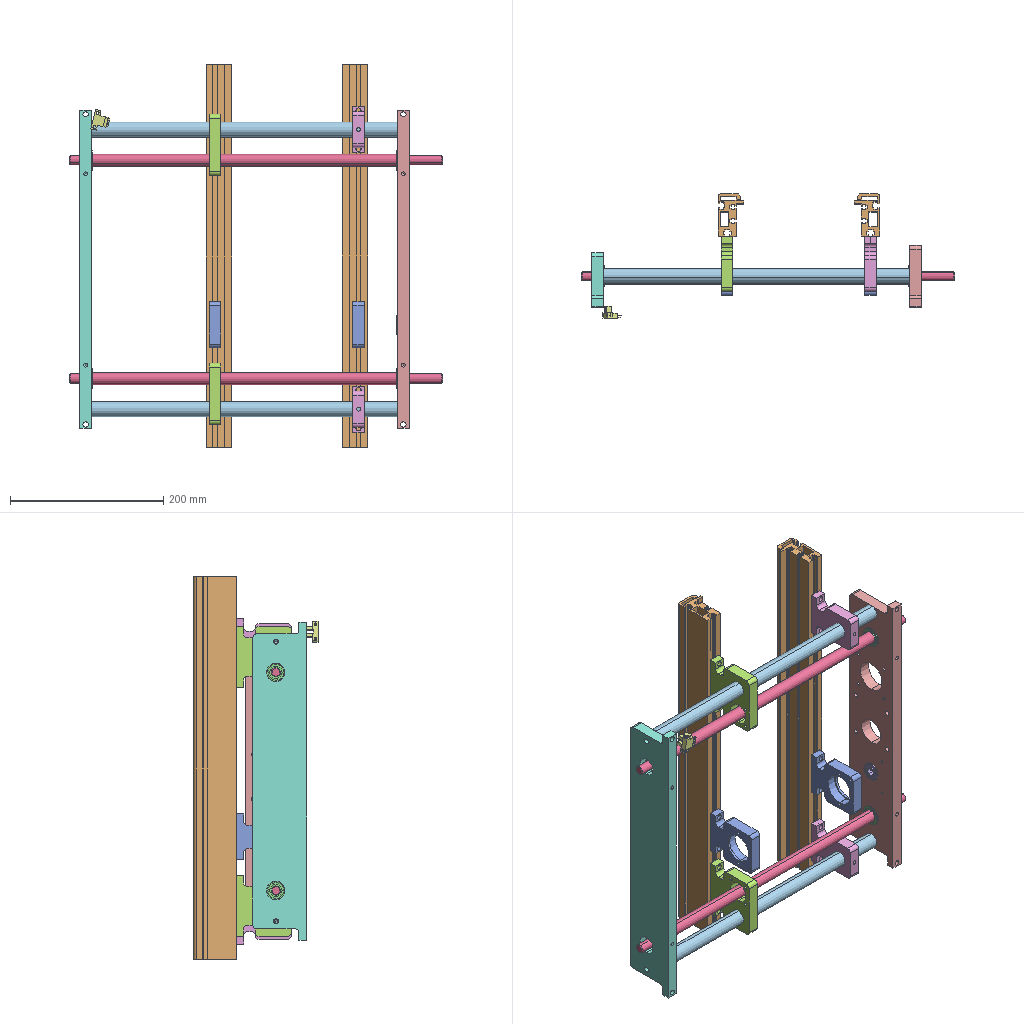Assembly | SolidWorks | 11 different items | 20 placed | box 487 x 162 x 500 mm
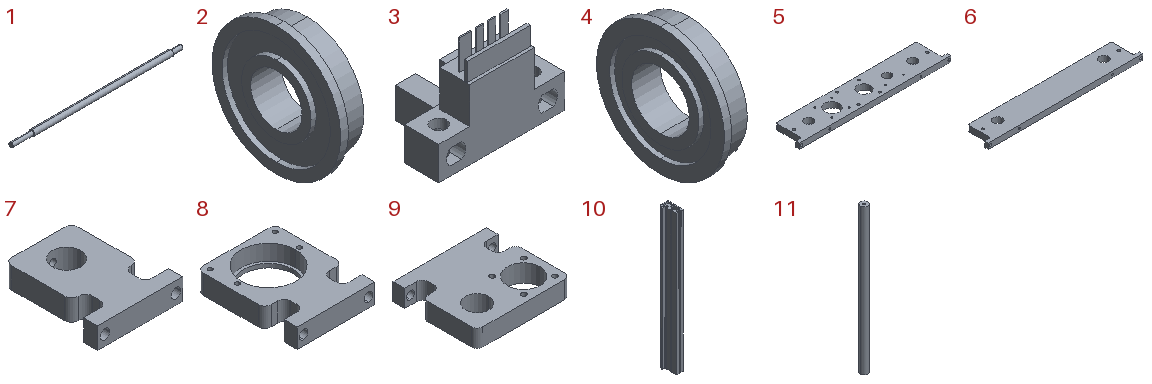Parts list (item | quantity | size | volume | features):
1 | x2 | 487 x 16 x 16 mm | 89965 mm3 | features ICE 4, Chamfer 2, Extrusion 1, Helix 1, SweepCut 1
2 | x1 | 6 x 25 x 25 mm | 1569 mm3 | features Stock 1
3 | x1 | 26.2 x 15.5 x 20.7 mm | 2180 mm3 | features BaseBody 1
4 | x4 | 6 x 26.5 x 26.5 mm | 1894 mm3 | features ICE 2, Revolution 1
5 | x1 | 415 x 80 x 15 mm | 408736 mm3 | features ICE 4, HoleWzd 3, Fillet 2, Extrusion 1
6 | x1 | 415 x 70 x 15 mm | 392754 mm3 | features Fillet 2, HoleWzd 2, ICE 2, Extrusion 1
7 | x2 | 60 x 72 x 15 mm | 42527 mm3 | features ICE 3, CirPattern 1, Extrusion 1, Fillet 1, HoleWzd 1
8 | x2 | 60 x 77 x 15 mm | 41283 mm3 | features ICE 3, HoleWzd 2, Extrusion 1, Fillet 1
9 | x2 | 80 x 72 x 15 mm | 64030 mm3 | features ICE 2, Extrusion 1, Fillet 1, HoleWzd 1, MoveCopyBody 1
10 | x2 | 33.5 x 55 x 500 mm | 409209 mm3 | features Extrusion 1, ICE 1
11 | x2 | 20 x 20 x 400 mm | 125055 mm3 | features HoleWzd 2, Extrusion 1
Mates (type | each side: item.copy, entity, surface, feature):
Concentric | 5.1 face cylinder Cut-Extrude1 | 8.1 face cylinder Cut-Extrude4
Parallel | 5.1 face plane Boss-Extrude1 | 8.1 face plane Boss-Extrude1
Concentric | 5.1 face cylinder Cut-Extrude1 | 9.1 face cylinder Cut-Extrude2 | 2 times
Concentric | 5.1 face cylinder Cut-Extrude1 | 7.1 face cylinder Cut-Extrude1
Coincident | 8.1 face plane Boss-Extrude1 | 7.1 face plane Boss-Extrude1 | 2 times
Concentric | 5.1 face cylinder Cut-Extrude1 | 9.2 face cylinder Cut-Extrude2 | 2 times
Coincident | 9.1 face plane Boss-Extrude1 | 9.2 face plane Boss-Extrude1
Concentric | 5.1 face cylinder Cut-Extrude1 | 7.2 face cylinder Cut-Extrude1
Coincident | 8.1 face plane Boss-Extrude1 | 7.2 face plane Boss-Extrude1 | 2 times
Concentric | 5.1 face cylinder Cut-Extrude1 | 8.2 face cylinder Cut-Extrude4
Coincident | 9.2 face plane Boss-Extrude1 | 8.2 face plane Boss-Extrude1 | 2 times
Coincident | 5.1 face plane Boss-Extrude1 | 6.1 face plane Boss-Extrude1
Concentric | 5.1 face cylinder Cut-Extrude1 | 6.1 face cylinder Cut-Extrude1 | 2 times
Coincident | 7.1 face plane Boss-Extrude1 | 10.1 face plane Boss-Extrude1
DistanceDim | 10.1 face plane Boss-Extrude1 | 7.1 face plane Boss-Extrude1
Coincident | 9.1 face plane Boss-Extrude1 | 10.2 face plane Boss-Extrude1
DistanceDim | 10.2 face plane Boss-Extrude1 | 9.1 face plane Boss-Extrude1
Coincident | 10.1 face plane Boss-Extrude1 | 10.2 face plane Boss-Extrude1
DistanceDim | 10.2 face plane Boss-Extrude1 | 5.1 face plane Boss-Extrude1
Concentric | 5.1 face cylinder Cut-Extrude1 | 4.1 face cylinder Revolve1
Coincident | 5.1 face plane Boss-Extrude1 | 4.1 face plane Revolve1
Concentric | 5.1 face cylinder Cut-Extrude1 | 2.1 face cylinder F6900Z Bearing
Coincident | 5.1 face plane Boss-Extrude1 | 2.1 face plane F6900Z Bearing
Concentric | 5.1 face cylinder Cut-Extrude1 | 4.2 face cylinder Revolve1
Coincident | 5.1 face plane Boss-Extrude1 | 4.2 face plane Revolve1
Concentric | 6.1 face cylinder Cut-Extrude1 | 4.3 face cylinder Revolve1
Coincident | 6.1 face plane Boss-Extrude1 | 4.3 face plane Revolve1
Concentric | 6.1 face cylinder Cut-Extrude1 | 4.4 face cylinder Revolve1
Coincident | 6.1 face plane Boss-Extrude1 | 4.4 face plane Revolve1
Concentric | 5.1 face cylinder Cut-Extrude1 | 1.1 face cylinder Boss-Extrude3
Coincident | 4.1 face plane Revolve1 | 1.1 face plane Boss-Extrude1
Concentric | 5.1 face cylinder Cut-Extrude1 | 1.2 face cylinder Boss-Extrude3
Coincident | 4.2 face plane Revolve1 | 1.2 face plane Boss-Extrude1
Concentric | 5.1 face cylinder Cut-Extrude1 | 11.1 face cylinder Boss-Extrude1
Coincident | 5.1 face plane Boss-Extrude1 | 11.1 face plane Boss-Extrude1
Concentric | 5.1 face cylinder Cut-Extrude1 | 11.2 face cylinder Boss-Extrude1
Coincident | 5.1 face plane Boss-Extrude1 | 11.2 face plane Boss-Extrude1
Coincident | 6.1 face plane Boss-Extrude1 | 11.2 face plane Boss-Extrude1
DistanceDim | 3.1 face plane Imported1 | 6.1 face plane Boss-Extrude1